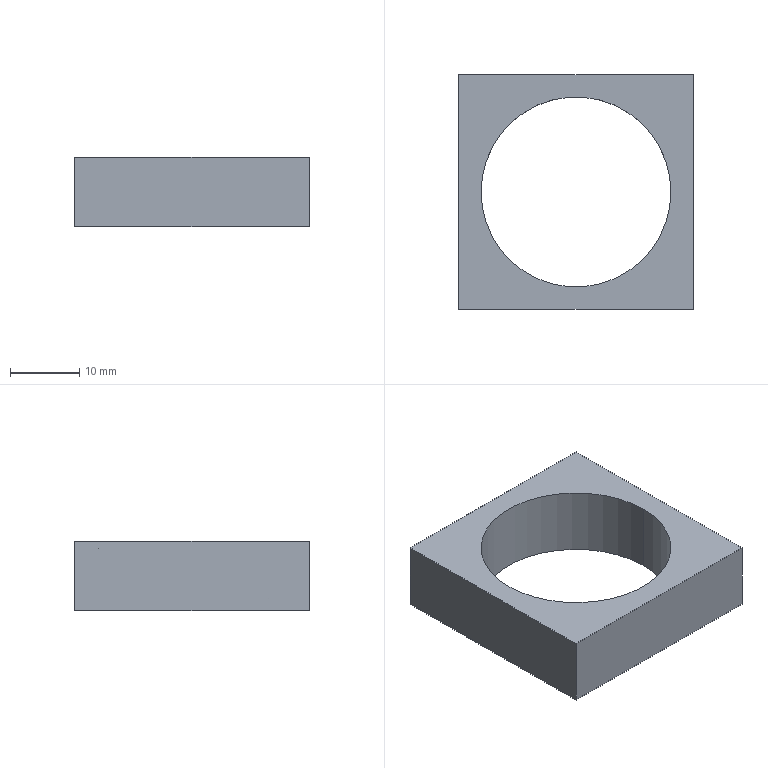Part | STEP file | X77-09110 | 1 solid | 8 faces | box 34 x 34 x 10 mm | volume 5620 mm3 | plane 6 | cylinder 2 | commonest cylinder face diameters 27.5 x2
STEP:
#1=CARTESIAN_POINT('',(-493.75,-20.,-10.));
#2=VERTEX_POINT('',#1);
#3=CARTESIAN_POINT('',(-466.25,-20.,-10.));
#4=VERTEX_POINT('',#3);
#5=CARTESIAN_POINT('',(-480.,-20.,-10.));
#6=DIRECTION('',(0.,0.,1.));
#7=DIRECTION('',(1.,0.,0.));
#8=AXIS2_PLACEMENT_3D('',#5,#6,#7);
#9=CIRCLE('',#8,13.75);
#10=EDGE_CURVE('',#2,#4,#9,.T.);
#11=ORIENTED_EDGE('',*,*,#10,.F.);
#12=CARTESIAN_POINT('',(-493.75,-20.,0.));
#13=VERTEX_POINT('',#12);
#14=CARTESIAN_POINT('',(-493.75,-20.,-10.));
#15=DIRECTION('',(0.,0.,1.));
#16=VECTOR('',#15,1000.);
#17=LINE('',#14,#16);
#18=EDGE_CURVE('',#2,#13,#17,.T.);
#19=ORIENTED_EDGE('',*,*,#18,.T.);
#20=CARTESIAN_POINT('',(-466.25,-20.,0.));
#21=VERTEX_POINT('',#20);
#22=CARTESIAN_POINT('',(-480.,-20.,0.));
#23=DIRECTION('',(0.,0.,1.));
#24=DIRECTION('',(1.,0.,0.));
#25=AXIS2_PLACEMENT_3D('',#22,#23,#24);
#26=CIRCLE('',#25,13.75);
#27=EDGE_CURVE('',#13,#21,#26,.T.);
#28=ORIENTED_EDGE('',*,*,#27,.T.);
#29=CARTESIAN_POINT('',(-466.25,-20.,-10.));
#30=DIRECTION('',(0.,0.,1.));
#31=VECTOR('',#30,1000.);
#32=LINE('',#29,#31);
#33=EDGE_CURVE('',#4,#21,#32,.T.);
#34=ORIENTED_EDGE('',*,*,#33,.F.);
#35=EDGE_LOOP('',(#11,#19,#28,#34));
#36=FACE_OUTER_BOUND('',#35,.T.);
#37=CARTESIAN_POINT('',(-480.,-20.,-10.));
#38=DIRECTION('',(0.,0.,1.));
#39=DIRECTION('',(1.,0.,0.));
#40=AXIS2_PLACEMENT_3D('',#37,#38,#39);
#41=CYLINDRICAL_SURFACE('',#40,13.75);
#42=ADVANCED_FACE('',(#36),#41,.F.);
#43=CARTESIAN_POINT('',(-497.,-3.,0.));
#44=VERTEX_POINT('',#43);
#45=CARTESIAN_POINT('',(-497.,-37.,0.));
#46=VERTEX_POINT('',#45);
#47=CARTESIAN_POINT('',(-497.,-37.,0.));
#48=DIRECTION('',(0.,-1.,0.));
#49=VECTOR('',#48,1000.);
#50=LINE('',#47,#49);
#51=EDGE_CURVE('',#44,#46,#50,.T.);
#52=ORIENTED_EDGE('',*,*,#51,.F.);
#53=CARTESIAN_POINT('',(-497.,-3.,-10.));
#54=VERTEX_POINT('',#53);
#55=CARTESIAN_POINT('',(-497.,-3.,-10.));
#56=DIRECTION('',(0.,0.,1.));
#57=VECTOR('',#56,1000.);
#58=LINE('',#55,#57);
#59=EDGE_CURVE('',#54,#44,#58,.T.);
#60=ORIENTED_EDGE('',*,*,#59,.F.);
#61=CARTESIAN_POINT('',(-497.,-37.,-10.));
#62=VERTEX_POINT('',#61);
#63=CARTESIAN_POINT('',(-497.,-37.,-10.));
#64=DIRECTION('',(0.,-1.,0.));
#65=VECTOR('',#64,1000.);
#66=LINE('',#63,#65);
#67=EDGE_CURVE('',#54,#62,#66,.T.);
#68=ORIENTED_EDGE('',*,*,#67,.T.);
#69=CARTESIAN_POINT('',(-497.,-37.,-10.));
#70=DIRECTION('',(0.,0.,1.));
#71=VECTOR('',#70,1000.);
#72=LINE('',#69,#71);
#73=EDGE_CURVE('',#62,#46,#72,.T.);
#74=ORIENTED_EDGE('',*,*,#73,.T.);
#75=EDGE_LOOP('',(#52,#60,#68,#74));
#76=FACE_OUTER_BOUND('',#75,.T.);
#77=CARTESIAN_POINT('',(-497.,-37.,-10.));
#78=DIRECTION('',(-1.,0.,0.));
#79=DIRECTION('',(0.,0.,1.));
#80=AXIS2_PLACEMENT_3D('',#77,#78,#79);
#81=PLANE('',#80);
#82=ADVANCED_FACE('',(#76),#81,.T.);
#83=CARTESIAN_POINT('',(-463.,-3.,0.));
#84=VERTEX_POINT('',#83);
#85=CARTESIAN_POINT('',(-497.,-3.,0.));
#86=DIRECTION('',(-1.,0.,0.));
#87=VECTOR('',#86,1000.);
#88=LINE('',#85,#87);
#89=EDGE_CURVE('',#84,#44,#88,.T.);
#90=ORIENTED_EDGE('',*,*,#89,.F.);
#91=CARTESIAN_POINT('',(-463.,-3.,-10.));
#92=VERTEX_POINT('',#91);
#93=CARTESIAN_POINT('',(-463.,-3.,-10.));
#94=DIRECTION('',(0.,0.,1.));
#95=VECTOR('',#94,1000.);
#96=LINE('',#93,#95);
#97=EDGE_CURVE('',#92,#84,#96,.T.);
#98=ORIENTED_EDGE('',*,*,#97,.F.);
#99=CARTESIAN_POINT('',(-497.,-3.,-10.));
#100=DIRECTION('',(-1.,0.,0.));
#101=VECTOR('',#100,1000.);
#102=LINE('',#99,#101);
#103=EDGE_CURVE('',#92,#54,#102,.T.);
#104=ORIENTED_EDGE('',*,*,#103,.T.);
#105=ORIENTED_EDGE('',*,*,#59,.T.);
#106=EDGE_LOOP('',(#90,#98,#104,#105));
#107=FACE_OUTER_BOUND('',#106,.T.);
#108=CARTESIAN_POINT('',(-497.,-3.,-10.));
#109=DIRECTION('',(0.,1.,0.));
#110=DIRECTION('',(0.,0.,1.));
#111=AXIS2_PLACEMENT_3D('',#108,#109,#110);
#112=PLANE('',#111);
#113=ADVANCED_FACE('',(#107),#112,.T.);
#114=CARTESIAN_POINT('',(-463.,-37.,0.));
#115=VERTEX_POINT('',#114);
#116=CARTESIAN_POINT('',(-463.,-37.,0.));
#117=DIRECTION('',(0.,1.,0.));
#118=VECTOR('',#117,1000.);
#119=LINE('',#116,#118);
#120=EDGE_CURVE('',#115,#84,#119,.T.);
#121=ORIENTED_EDGE('',*,*,#120,.F.);
#122=CARTESIAN_POINT('',(-463.,-37.,-10.));
#123=VERTEX_POINT('',#122);
#124=CARTESIAN_POINT('',(-463.,-37.,-10.));
#125=DIRECTION('',(0.,0.,1.));
#126=VECTOR('',#125,1000.);
#127=LINE('',#124,#126);
#128=EDGE_CURVE('',#123,#115,#127,.T.);
#129=ORIENTED_EDGE('',*,*,#128,.F.);
#130=CARTESIAN_POINT('',(-463.,-37.,-10.));
#131=DIRECTION('',(0.,1.,0.));
#132=VECTOR('',#131,1000.);
#133=LINE('',#130,#132);
#134=EDGE_CURVE('',#123,#92,#133,.T.);
#135=ORIENTED_EDGE('',*,*,#134,.T.);
#136=ORIENTED_EDGE('',*,*,#97,.T.);
#137=EDGE_LOOP('',(#121,#129,#135,#136));
#138=FACE_OUTER_BOUND('',#137,.T.);
#139=CARTESIAN_POINT('',(-463.,-37.,-10.));
#140=DIRECTION('',(1.,0.,0.));
#141=DIRECTION('',(0.,0.,-1.));
#142=AXIS2_PLACEMENT_3D('',#139,#140,#141);
#143=PLANE('',#142);
#144=ADVANCED_FACE('',(#138),#143,.T.);
#145=CARTESIAN_POINT('',(-497.,-37.,0.));
#146=DIRECTION('',(1.,0.,0.));
#147=VECTOR('',#146,1000.);
#148=LINE('',#145,#147);
#149=EDGE_CURVE('',#46,#115,#148,.T.);
#150=ORIENTED_EDGE('',*,*,#149,.F.);
#151=ORIENTED_EDGE('',*,*,#73,.F.);
#152=CARTESIAN_POINT('',(-497.,-37.,-10.));
#153=DIRECTION('',(1.,0.,0.));
#154=VECTOR('',#153,1000.);
#155=LINE('',#152,#154);
#156=EDGE_CURVE('',#62,#123,#155,.T.);
#157=ORIENTED_EDGE('',*,*,#156,.T.);
#158=ORIENTED_EDGE('',*,*,#128,.T.);
#159=EDGE_LOOP('',(#150,#151,#157,#158));
#160=FACE_OUTER_BOUND('',#159,.T.);
#161=CARTESIAN_POINT('',(-497.,-37.,-10.));
#162=DIRECTION('',(0.,-1.,0.));
#163=DIRECTION('',(0.,0.,-1.));
#164=AXIS2_PLACEMENT_3D('',#161,#162,#163);
#165=PLANE('',#164);
#166=ADVANCED_FACE('',(#160),#165,.T.);
#167=CARTESIAN_POINT('',(-480.,-20.,-10.));
#168=DIRECTION('',(0.,0.,1.));
#169=DIRECTION('',(1.,0.,0.));
#170=AXIS2_PLACEMENT_3D('',#167,#168,#169);
#171=CIRCLE('',#170,13.75);
#172=EDGE_CURVE('',#4,#2,#171,.T.);
#173=ORIENTED_EDGE('',*,*,#172,.T.);
#174=ORIENTED_EDGE('',*,*,#10,.T.);
#175=EDGE_LOOP('',(#173,#174));
#176=FACE_BOUND('',#175,.T.);
#177=ORIENTED_EDGE('',*,*,#67,.F.);
#178=ORIENTED_EDGE('',*,*,#103,.F.);
#179=ORIENTED_EDGE('',*,*,#134,.F.);
#180=ORIENTED_EDGE('',*,*,#156,.F.);
#181=EDGE_LOOP('',(#177,#178,#179,#180));
#182=FACE_OUTER_BOUND('',#181,.T.);
#183=CARTESIAN_POINT('',(-497.,-3.,-10.));
#184=DIRECTION('',(0.,0.,-1.));
#185=DIRECTION('',(-1.,0.,0.));
#186=AXIS2_PLACEMENT_3D('',#183,#184,#185);
#187=PLANE('',#186);
#188=ADVANCED_FACE('',(#176,#182),#187,.T.);
#189=CARTESIAN_POINT('',(-480.,-20.,0.));
#190=DIRECTION('',(0.,0.,1.));
#191=DIRECTION('',(1.,0.,0.));
#192=AXIS2_PLACEMENT_3D('',#189,#190,#191);
#193=CIRCLE('',#192,13.75);
#194=EDGE_CURVE('',#21,#13,#193,.T.);
#195=ORIENTED_EDGE('',*,*,#194,.F.);
#196=ORIENTED_EDGE('',*,*,#27,.F.);
#197=EDGE_LOOP('',(#195,#196));
#198=FACE_BOUND('',#197,.T.);
#199=ORIENTED_EDGE('',*,*,#51,.T.);
#200=ORIENTED_EDGE('',*,*,#149,.T.);
#201=ORIENTED_EDGE('',*,*,#120,.T.);
#202=ORIENTED_EDGE('',*,*,#89,.T.);
#203=EDGE_LOOP('',(#199,#200,#201,#202));
#204=FACE_OUTER_BOUND('',#203,.T.);
#205=CARTESIAN_POINT('',(-497.,-3.,0.));
#206=DIRECTION('',(0.,0.,-1.));
#207=DIRECTION('',(-1.,0.,0.));
#208=AXIS2_PLACEMENT_3D('',#205,#206,#207);
#209=PLANE('',#208);
#210=ADVANCED_FACE('',(#198,#204),#209,.F.);
#211=ORIENTED_EDGE('',*,*,#18,.F.);
#212=ORIENTED_EDGE('',*,*,#172,.F.);
#213=ORIENTED_EDGE('',*,*,#33,.T.);
#214=ORIENTED_EDGE('',*,*,#194,.T.);
#215=EDGE_LOOP('',(#211,#212,#213,#214));
#216=FACE_OUTER_BOUND('',#215,.T.);
#217=CARTESIAN_POINT('',(-480.,-20.,-10.));
#218=DIRECTION('',(0.,0.,1.));
#219=DIRECTION('',(1.,0.,0.));
#220=AXIS2_PLACEMENT_3D('',#217,#218,#219);
#221=CYLINDRICAL_SURFACE('',#220,13.75);
#222=ADVANCED_FACE('',(#216),#221,.F.);
#223=CLOSED_SHELL('',(#42,#82,#113,#144,#166,#188,#210,#222));
#224=MANIFOLD_SOLID_BREP('',#223);
#225=CARTESIAN_POINT('',(0.,0.,0.));
#226=DIRECTION('',(0.,0.,1.));
#227=DIRECTION('',(1.,0.,0.));
#228=AXIS2_PLACEMENT_3D('',#225,#226,#227);
#229=(LENGTH_UNIT()NAMED_UNIT(*)SI_UNIT(.MILLI.,.METRE.));
#230=UNCERTAINTY_MEASURE_WITH_UNIT(LENGTH_MEASURE(0.00001),#229,'','');
#231=(NAMED_UNIT(*)PLANE_ANGLE_UNIT()SI_UNIT($,.RADIAN.));
#232=(NAMED_UNIT(*)SI_UNIT($,.STERADIAN.)SOLID_ANGLE_UNIT());
#233=(GEOMETRIC_REPRESENTATION_CONTEXT(3)GLOBAL_UNCERTAINTY_ASSIGNED_CONTEXT((#230))GLOBAL_UNIT_ASSIGNED_CONTEXT((#229,#231,#232))REPRESENTATION_CONTEXT('',''));
#234=ADVANCED_BREP_SHAPE_REPRESENTATION('',(#224,#228),#233);